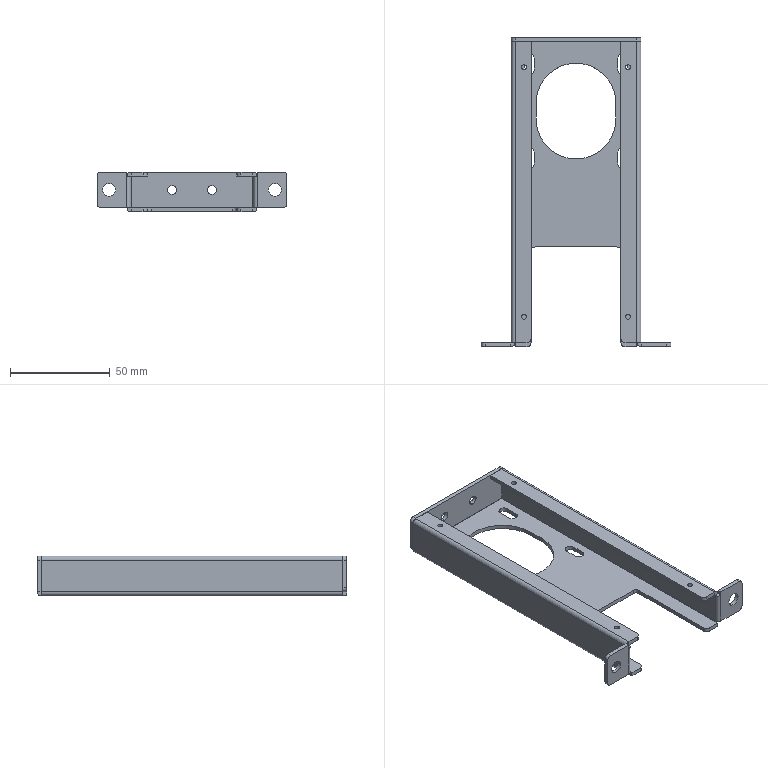Part | STEP file | 1 solid | 120 faces | box 95 x 155 x 20 mm | volume 30386 mm3 | plane 68 | cylinder 52 | commonest cylinder face diameters 4 x12 2.5 x8 5 x8 0.2 x7 4.2 x7 4.5 x4